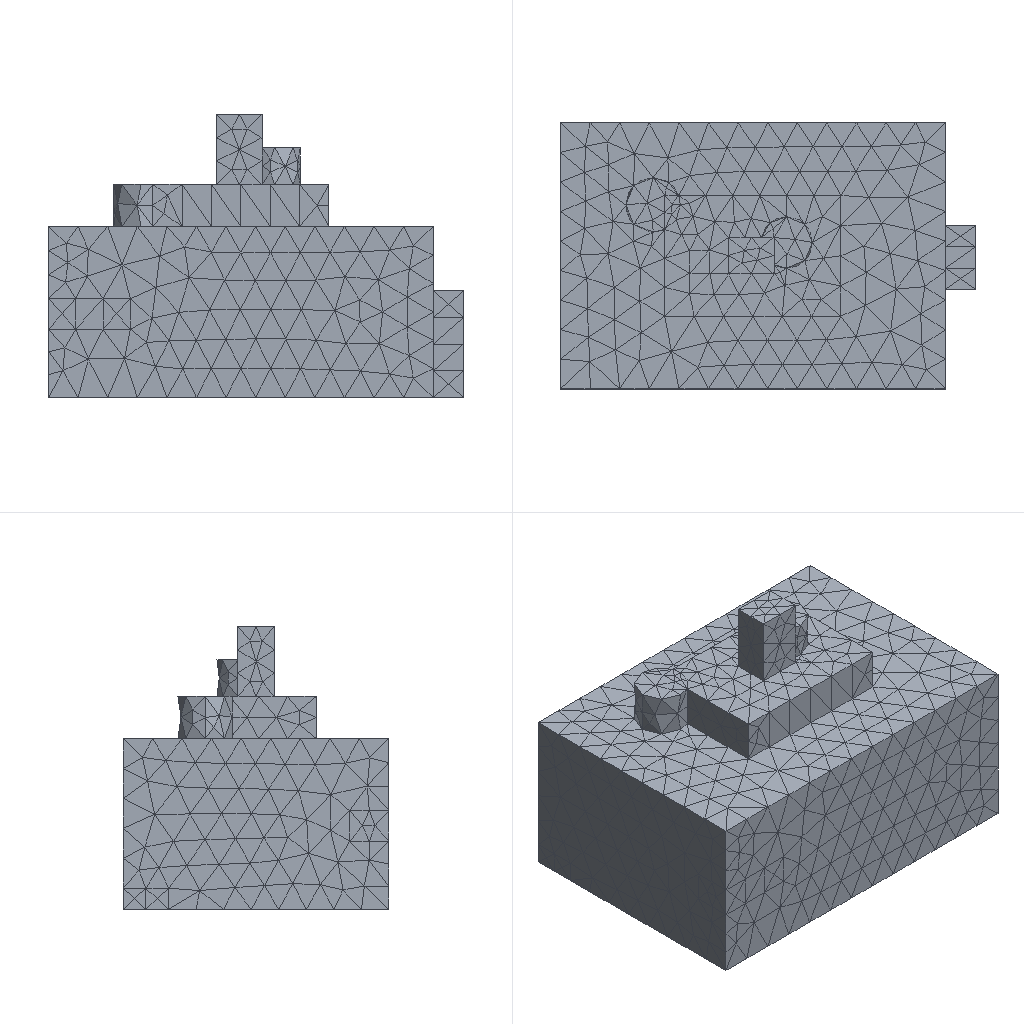Simulation study | ansys mapdl
Set-up summary:
category,name,step,type,value,unit,region
solver,ansys_mapdl
units,mm-N-s-tonne (MPa),,inferred,E=210000 density=
analysis,model,,static
mesh,nodes,,,11454
mesh,elements,,,7373
element_type,SOLID187,,,7373
material,mat 1,,E,210000
material,mat 1,,nu,0.3
load,,model,body load temp,,,all
load,,model,force,"1000 [dir=(0, 0, -1) n=351]",,node list
bc,,model,fixed,"[dofs=UX,UY,UZ n=11886]",,node list
Ansys APDL input file, long lists of numbers shortened:
/COM,ANSYS RELEASE 2026 R1           BUILD 26.1      UP20260202       09:08:29
/PREP7
/NOPR
/TITLE,2
ANTYPE, 0
*IF,_CDRDOFF,EQ,1,THEN     !if solid model was read in
_CDRDOFF=             !reset flag, numoffs already performed
*ELSE              !offset database for the following FE model
NUMOFF,NODE,    11454
NUMOFF,ELEM,     7373
NUMOFF,MAT ,        1
NUMOFF,TYPE,        1
*ENDIF
*SET,_RETURN ,  0.
*SET,_STATUS ,  0.
*SET,_UIQR   ,  351.
*SET,__FLOATPARAMETER__,  11454.
DOF,DELETE
ETBLOCK,        1,        1
(2i9,19a9)
        1      187        0        0        0        0        0        0        0        0        0        0        0        0        0        0        0        0        0        0        0
       -1
NBLOCK,6,SOLID,     11454,     11454
(3i9,6e21.13e3)
        1        0        0 7.0000000000000E+000 6.0000000000000E+000 9.3390000000000E+001
! (11453 more lines like these left out)
N,UNBL,LOC,       -1,
EBLOCK,19,SOLID,      7373,      7373
(19i10)
         1         1         1         1         0         0         0         0        10         0         1      3147      3148      3149      3150      4007      4008      4009      4010
! (14745 more lines like these left out)
        -1
MPTEMP,UNBL, 1, 1,  0.    ,
MPDATA,UNBL, 1,EX  ,       1, 1,  210000.000    ,
MPTEMP,UNBL, 1, 1,  0.    ,
MPDATA,UNBL, 1,NUXY,       1, 1, 0.3    ,
MPTEMP,UNBL, 1, 1,  0.    ,
MPDATA,UNBL, 1,PRXY,       1, 1, 0.3    ,
EXTOPT,ATTR,      0,      0,      0
EXTOPT,ESIZE,  0,  0.
EXTOPT,ACLEAR,      0
TREF,  0.
IRLF,  0
BFUNIF,TEMP,_TINY
ACEL,  0.    ,  0.    ,  0.
OMEGA,  0.    ,  0.    ,  0.
DOMEGA,  0.    ,  0.    ,  0.
CGLOC,  0.    ,  0.    ,  0.
CGOMEGA,  0.    ,  0.    ,  0.
DCGOMG,  0.    ,  0.    ,  0.
KUSE,     0
TIME,  0.
ALPHAD,  0.
BETAD,  0.
DMPRAT,  0.
DMPSTR,  0.
CRPLIM, 0.1    ,   0
CRPLIM,  0.    ,   1
NCNV,     0, 1.000000000E+12,     0,  0.    ,  0.
NEQIT,     0
ERESX,DEFA
DBLOCK,     11886
(i9,a6,2(pg16.9))
      551  UX    0.00000000      0.00000000
! (11885 more lines like these left out)
       -1
FBLOCK,       351
(i9,a6,2(pg16.9))
        1  FZ   -2.84900285      0.00000000
! (350 more lines like these left out)
       -1
/GO
FINISH
Results summary:
result,analysis_type_db,,,static,unstated
result,n_sets,,,1,unstated
result,load_steps[0].set,load_step=1,,1,unstated
result,load_steps[0].substep,load_step=1,,1,unstated
result,load_steps[0].time,load_step=1,,1,unstated
result,load_steps[0].freq,load_step=1,,1,unstated
result,load_steps[0].max_usum,load_step=1,,0.0005314,unstated
result,load_steps[0].max_seqv,load_step=1,,4.334,unstated
result,load_steps[0].reaction_sum.FX,load_step=1,,-6.46772e-11,unstated
result,load_steps[0].reaction_sum.FY,load_step=1,,2.26184e-11,unstated
result,load_steps[0].reaction_sum.FZ,load_step=1,,1000,unstated
result,load_steps[0].reaction_sum.MX,load_step=1,,0,unstated
result,load_steps[0].reaction_sum.MY,load_step=1,,0,unstated
result,load_steps[0].reaction_sum.MZ,load_step=1,,0,unstated
result,convergence,,,results present for all listed sets,unstated